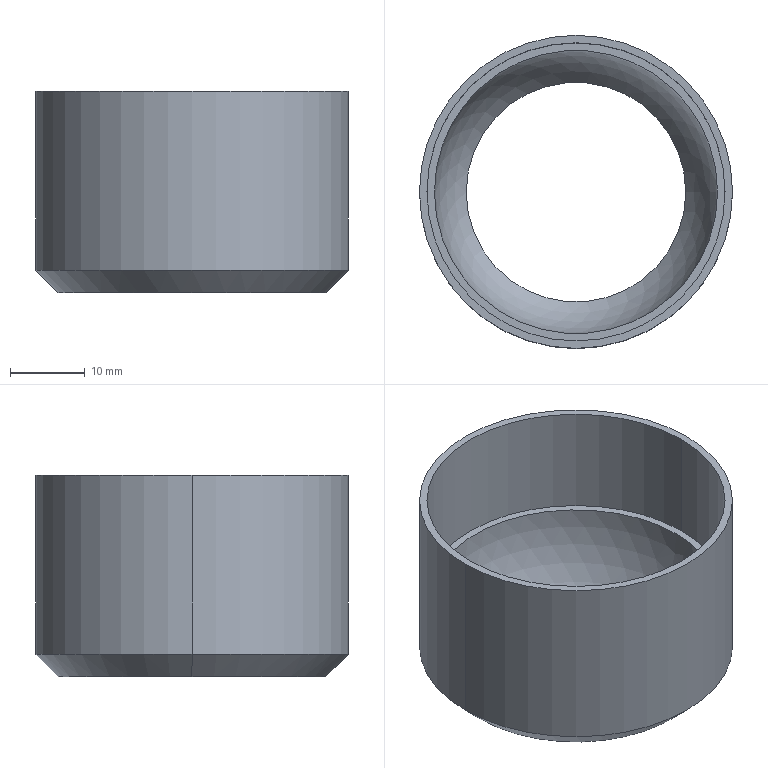Part | SolidWorks | features ICE 5, Chamfer 1, Extrusion 1, RevCut 1 | 1 solid | 10 faces | box 42 x 42 x 27 mm | volume 6192 mm3 | cylinder 4 | plane 3 | cone 2 | sphere 1 | commonest cylinder face diameters 40 x2 42 x2
STEP:
#1=CARTESIAN_POINT('',(-18.,0.,18.));
#2=VERTEX_POINT('',#1);
#3=CARTESIAN_POINT('',(18.,0.,18.));
#4=VERTEX_POINT('',#3);
#5=CARTESIAN_POINT('',(0.,0.,18.));
#6=DIRECTION('',(0.,0.,-1.));
#7=DIRECTION('',(-1.,0.,0.));
#8=AXIS2_PLACEMENT_3D('',#5,#6,#7);
#9=CIRCLE('',#8,18.);
#10=EDGE_CURVE('',#2,#4,#9,.T.);
#11=ORIENTED_EDGE('',*,*,#10,.F.);
#12=CARTESIAN_POINT('',(-21.,0.,21.));
#13=VERTEX_POINT('',#12);
#14=CARTESIAN_POINT('',(-18.,0.,18.));
#15=DIRECTION('',(-0.7071,0.,0.7071));
#16=VECTOR('',#15,1000.);
#17=LINE('',#14,#16);
#18=EDGE_CURVE('',#2,#13,#17,.T.);
#19=ORIENTED_EDGE('',*,*,#18,.T.);
#20=CARTESIAN_POINT('',(21.,0.,21.));
#21=VERTEX_POINT('',#20);
#22=CARTESIAN_POINT('',(0.,0.,21.));
#23=DIRECTION('',(0.,0.,1.));
#24=DIRECTION('',(-1.,0.,0.));
#25=AXIS2_PLACEMENT_3D('',#22,#23,#24);
#26=CIRCLE('',#25,21.);
#27=EDGE_CURVE('',#21,#13,#26,.T.);
#28=ORIENTED_EDGE('',*,*,#27,.F.);
#29=CARTESIAN_POINT('',(18.,0.,18.));
#30=DIRECTION('',(0.7071,0.,0.7071));
#31=VECTOR('',#30,1000.);
#32=LINE('',#29,#31);
#33=EDGE_CURVE('',#4,#21,#32,.T.);
#34=ORIENTED_EDGE('',*,*,#33,.F.);
#35=EDGE_LOOP('',(#11,#19,#28,#34));
#36=FACE_OUTER_BOUND('',#35,.T.);
#37=CARTESIAN_POINT('',(0.,0.,18.));
#38=DIRECTION('',(0.,0.,1.));
#39=DIRECTION('',(1.,0.,0.));
#40=AXIS2_PLACEMENT_3D('',#37,#38,#39);
#41=CONICAL_SURFACE('',#40,18.,0.7854);
#42=ADVANCED_FACE('',(#36),#41,.T.);
#43=CARTESIAN_POINT('',(-20.,0.,30.));
#44=VERTEX_POINT('',#43);
#45=CARTESIAN_POINT('',(20.,0.,30.));
#46=VERTEX_POINT('',#45);
#47=CARTESIAN_POINT('',(0.,0.,30.));
#48=DIRECTION('',(0.,0.,1.));
#49=DIRECTION('',(1.,0.,0.));
#50=AXIS2_PLACEMENT_3D('',#47,#48,#49);
#51=CIRCLE('',#50,20.);
#52=EDGE_CURVE('',#44,#46,#51,.T.);
#53=ORIENTED_EDGE('',*,*,#52,.F.);
#54=CARTESIAN_POINT('',(-20.,0.,45.));
#55=VERTEX_POINT('',#54);
#56=CARTESIAN_POINT('',(-20.,0.,30.));
#57=DIRECTION('',(0.,0.,1.));
#58=VECTOR('',#57,1000.);
#59=LINE('',#56,#58);
#60=EDGE_CURVE('',#44,#55,#59,.T.);
#61=ORIENTED_EDGE('',*,*,#60,.T.);
#62=CARTESIAN_POINT('',(20.,0.,45.));
#63=VERTEX_POINT('',#62);
#64=CARTESIAN_POINT('',(0.,0.,45.));
#65=DIRECTION('',(0.,0.,1.));
#66=DIRECTION('',(1.,0.,0.));
#67=AXIS2_PLACEMENT_3D('',#64,#65,#66);
#68=CIRCLE('',#67,20.);
#69=EDGE_CURVE('',#55,#63,#68,.T.);
#70=ORIENTED_EDGE('',*,*,#69,.T.);
#71=CARTESIAN_POINT('',(20.,0.,30.));
#72=DIRECTION('',(0.,0.,1.));
#73=VECTOR('',#72,1000.);
#74=LINE('',#71,#73);
#75=EDGE_CURVE('',#46,#63,#74,.T.);
#76=ORIENTED_EDGE('',*,*,#75,.F.);
#77=EDGE_LOOP('',(#53,#61,#70,#76));
#78=FACE_OUTER_BOUND('',#77,.T.);
#79=CARTESIAN_POINT('',(0.,0.,30.));
#80=DIRECTION('',(0.,0.,1.));
#81=DIRECTION('',(1.,0.,0.));
#82=AXIS2_PLACEMENT_3D('',#79,#80,#81);
#83=CYLINDRICAL_SURFACE('',#82,20.);
#84=ADVANCED_FACE('',(#78),#83,.F.);
#85=CARTESIAN_POINT('',(21.,0.,45.));
#86=VERTEX_POINT('',#85);
#87=CARTESIAN_POINT('',(-21.,0.,45.));
#88=VERTEX_POINT('',#87);
#89=CARTESIAN_POINT('',(0.,0.,45.));
#90=DIRECTION('',(0.,0.,1.));
#91=DIRECTION('',(1.,0.,0.));
#92=AXIS2_PLACEMENT_3D('',#89,#90,#91);
#93=CIRCLE('',#92,21.);
#94=EDGE_CURVE('',#86,#88,#93,.T.);
#95=ORIENTED_EDGE('',*,*,#94,.F.);
#96=CARTESIAN_POINT('',(21.,0.,45.));
#97=DIRECTION('',(0.,0.,-1.));
#98=VECTOR('',#97,1000.);
#99=LINE('',#96,#98);
#100=EDGE_CURVE('',#86,#21,#99,.T.);
#101=ORIENTED_EDGE('',*,*,#100,.T.);
#102=ORIENTED_EDGE('',*,*,#27,.T.);
#103=CARTESIAN_POINT('',(-21.,0.,45.));
#104=DIRECTION('',(0.,0.,-1.));
#105=VECTOR('',#104,1000.);
#106=LINE('',#103,#105);
#107=EDGE_CURVE('',#88,#13,#106,.T.);
#108=ORIENTED_EDGE('',*,*,#107,.F.);
#109=EDGE_LOOP('',(#95,#101,#102,#108));
#110=FACE_OUTER_BOUND('',#109,.T.);
#111=CARTESIAN_POINT('',(0.,0.,45.));
#112=DIRECTION('',(0.,0.,-1.));
#113=DIRECTION('',(-1.,0.,0.));
#114=AXIS2_PLACEMENT_3D('',#111,#112,#113);
#115=CYLINDRICAL_SURFACE('',#114,21.);
#116=ADVANCED_FACE('',(#110),#115,.T.);
#117=ORIENTED_EDGE('',*,*,#100,.F.);
#118=CARTESIAN_POINT('',(0.,0.,45.));
#119=DIRECTION('',(0.,0.,1.));
#120=DIRECTION('',(1.,0.,0.));
#121=AXIS2_PLACEMENT_3D('',#118,#119,#120);
#122=CIRCLE('',#121,21.);
#123=EDGE_CURVE('',#88,#86,#122,.T.);
#124=ORIENTED_EDGE('',*,*,#123,.F.);
#125=ORIENTED_EDGE('',*,*,#107,.T.);
#126=CARTESIAN_POINT('',(0.,0.,21.));
#127=DIRECTION('',(0.,0.,1.));
#128=DIRECTION('',(-1.,0.,0.));
#129=AXIS2_PLACEMENT_3D('',#126,#127,#128);
#130=CIRCLE('',#129,21.);
#131=EDGE_CURVE('',#13,#21,#130,.T.);
#132=ORIENTED_EDGE('',*,*,#131,.T.);
#133=EDGE_LOOP('',(#117,#124,#125,#132));
#134=FACE_OUTER_BOUND('',#133,.T.);
#135=CARTESIAN_POINT('',(0.,0.,45.));
#136=DIRECTION('',(0.,0.,-1.));
#137=DIRECTION('',(-1.,0.,0.));
#138=AXIS2_PLACEMENT_3D('',#135,#136,#137);
#139=CYLINDRICAL_SURFACE('',#138,21.);
#140=ADVANCED_FACE('',(#134),#139,.T.);
#141=CARTESIAN_POINT('',(19.,0.,30.));
#142=VERTEX_POINT('',#141);
#143=CARTESIAN_POINT('',(-19.,0.,30.));
#144=VERTEX_POINT('',#143);
#145=CARTESIAN_POINT('',(0.,0.,30.));
#146=DIRECTION('',(0.,0.,-1.));
#147=DIRECTION('',(1.,0.,0.));
#148=AXIS2_PLACEMENT_3D('',#145,#146,#147);
#149=CIRCLE('',#148,19.);
#150=EDGE_CURVE('',#142,#144,#149,.T.);
#151=ORIENTED_EDGE('',*,*,#150,.F.);
#152=CARTESIAN_POINT('',(0.,0.,30.));
#153=DIRECTION('',(0.,0.,-1.));
#154=DIRECTION('',(1.,0.,0.));
#155=AXIS2_PLACEMENT_3D('',#152,#153,#154);
#156=CIRCLE('',#155,19.);
#157=EDGE_CURVE('',#144,#142,#156,.T.);
#158=ORIENTED_EDGE('',*,*,#157,.F.);
#159=EDGE_LOOP('',(#151,#158));
#160=FACE_OUTER_BOUND('',#159,.T.);
#161=CARTESIAN_POINT('',(-14.731,0.,18.));
#162=VERTEX_POINT('',#161);
#163=CARTESIAN_POINT('',(14.731,0.,18.));
#164=VERTEX_POINT('',#163);
#165=CARTESIAN_POINT('',(0.,0.,18.));
#166=DIRECTION('',(0.,0.,1.));
#167=DIRECTION('',(-1.,0.,0.));
#168=AXIS2_PLACEMENT_3D('',#165,#166,#167);
#169=CIRCLE('',#168,14.731);
#170=EDGE_CURVE('',#162,#164,#169,.T.);
#171=ORIENTED_EDGE('',*,*,#170,.F.);
#172=CARTESIAN_POINT('',(0.,0.,18.));
#173=DIRECTION('',(0.,0.,1.));
#174=DIRECTION('',(-1.,0.,0.));
#175=AXIS2_PLACEMENT_3D('',#172,#173,#174);
#176=CIRCLE('',#175,14.731);
#177=EDGE_CURVE('',#164,#162,#176,.T.);
#178=ORIENTED_EDGE('',*,*,#177,.F.);
#179=EDGE_LOOP('',(#171,#178));
#180=FACE_BOUND('',#179,.T.);
#181=CARTESIAN_POINT('',(0.,0.,30.));
#182=DIRECTION('',(0.,0.,-1.));
#183=DIRECTION('',(0.,-1.,0.));
#184=AXIS2_PLACEMENT_3D('',#181,#182,#183);
#185=SPHERICAL_SURFACE('',#184,19.);
#186=ADVANCED_FACE('',(#160,#180),#185,.F.);
#187=CARTESIAN_POINT('',(0.,0.,45.));
#188=DIRECTION('',(0.,0.,1.));
#189=DIRECTION('',(1.,0.,0.));
#190=AXIS2_PLACEMENT_3D('',#187,#188,#189);
#191=CIRCLE('',#190,20.);
#192=EDGE_CURVE('',#63,#55,#191,.T.);
#193=ORIENTED_EDGE('',*,*,#192,.F.);
#194=ORIENTED_EDGE('',*,*,#69,.F.);
#195=EDGE_LOOP('',(#193,#194));
#196=FACE_BOUND('',#195,.T.);
#197=ORIENTED_EDGE('',*,*,#123,.T.);
#198=ORIENTED_EDGE('',*,*,#94,.T.);
#199=EDGE_LOOP('',(#197,#198));
#200=FACE_OUTER_BOUND('',#199,.T.);
#201=CARTESIAN_POINT('',(0.,0.,45.));
#202=DIRECTION('',(0.,0.,1.));
#203=DIRECTION('',(1.,0.,0.));
#204=AXIS2_PLACEMENT_3D('',#201,#202,#203);
#205=PLANE('',#204);
#206=ADVANCED_FACE('',(#196,#200),#205,.T.);
#207=CARTESIAN_POINT('',(0.,0.,30.));
#208=DIRECTION('',(0.,0.,1.));
#209=DIRECTION('',(1.,0.,0.));
#210=AXIS2_PLACEMENT_3D('',#207,#208,#209);
#211=CIRCLE('',#210,20.);
#212=EDGE_CURVE('',#46,#44,#211,.T.);
#213=ORIENTED_EDGE('',*,*,#212,.T.);
#214=ORIENTED_EDGE('',*,*,#52,.T.);
#215=EDGE_LOOP('',(#213,#214));
#216=FACE_OUTER_BOUND('',#215,.T.);
#217=ORIENTED_EDGE('',*,*,#150,.T.);
#218=ORIENTED_EDGE('',*,*,#157,.T.);
#219=EDGE_LOOP('',(#217,#218));
#220=FACE_BOUND('',#219,.T.);
#221=CARTESIAN_POINT('',(0.,0.,30.));
#222=DIRECTION('',(0.,0.,1.));
#223=DIRECTION('',(1.,0.,0.));
#224=AXIS2_PLACEMENT_3D('',#221,#222,#223);
#225=PLANE('',#224);
#226=ADVANCED_FACE('',(#216,#220),#225,.T.);
#227=ORIENTED_EDGE('',*,*,#60,.F.);
#228=ORIENTED_EDGE('',*,*,#212,.F.);
#229=ORIENTED_EDGE('',*,*,#75,.T.);
#230=ORIENTED_EDGE('',*,*,#192,.T.);
#231=EDGE_LOOP('',(#227,#228,#229,#230));
#232=FACE_OUTER_BOUND('',#231,.T.);
#233=CARTESIAN_POINT('',(0.,0.,30.));
#234=DIRECTION('',(0.,0.,1.));
#235=DIRECTION('',(1.,0.,0.));
#236=AXIS2_PLACEMENT_3D('',#233,#234,#235);
#237=CYLINDRICAL_SURFACE('',#236,20.);
#238=ADVANCED_FACE('',(#232),#237,.F.);
#239=CARTESIAN_POINT('',(0.,0.,18.));
#240=DIRECTION('',(0.,0.,-1.));
#241=DIRECTION('',(-1.,0.,0.));
#242=AXIS2_PLACEMENT_3D('',#239,#240,#241);
#243=CIRCLE('',#242,18.);
#244=EDGE_CURVE('',#4,#2,#243,.T.);
#245=ORIENTED_EDGE('',*,*,#244,.T.);
#246=ORIENTED_EDGE('',*,*,#10,.T.);
#247=EDGE_LOOP('',(#245,#246));
#248=FACE_OUTER_BOUND('',#247,.T.);
#249=ORIENTED_EDGE('',*,*,#170,.T.);
#250=ORIENTED_EDGE('',*,*,#177,.T.);
#251=EDGE_LOOP('',(#249,#250));
#252=FACE_BOUND('',#251,.T.);
#253=CARTESIAN_POINT('',(0.,0.,18.));
#254=DIRECTION('',(0.,0.,-1.));
#255=DIRECTION('',(-1.,0.,0.));
#256=AXIS2_PLACEMENT_3D('',#253,#254,#255);
#257=PLANE('',#256);
#258=ADVANCED_FACE('',(#248,#252),#257,.T.);
#259=ORIENTED_EDGE('',*,*,#18,.F.);
#260=ORIENTED_EDGE('',*,*,#244,.F.);
#261=ORIENTED_EDGE('',*,*,#33,.T.);
#262=ORIENTED_EDGE('',*,*,#131,.F.);
#263=EDGE_LOOP('',(#259,#260,#261,#262));
#264=FACE_OUTER_BOUND('',#263,.T.);
#265=CARTESIAN_POINT('',(0.,0.,18.));
#266=DIRECTION('',(0.,0.,1.));
#267=DIRECTION('',(1.,0.,0.));
#268=AXIS2_PLACEMENT_3D('',#265,#266,#267);
#269=CONICAL_SURFACE('',#268,18.,0.7854);
#270=ADVANCED_FACE('',(#264),#269,.T.);
#271=CLOSED_SHELL('',(#42,#84,#116,#140,#186,#206,#226,#238,#258,#270));
#272=MANIFOLD_SOLID_BREP('',#271);
#273=CARTESIAN_POINT('',(0.,0.,0.));
#274=DIRECTION('',(0.,0.,1.));
#275=DIRECTION('',(1.,0.,0.));
#276=AXIS2_PLACEMENT_3D('',#273,#274,#275);
#277=(LENGTH_UNIT()NAMED_UNIT(*)SI_UNIT(.MILLI.,.METRE.));
#278=UNCERTAINTY_MEASURE_WITH_UNIT(LENGTH_MEASURE(0.00001),#277,'','');
#279=(NAMED_UNIT(*)PLANE_ANGLE_UNIT()SI_UNIT($,.RADIAN.));
#280=(NAMED_UNIT(*)SI_UNIT($,.STERADIAN.)SOLID_ANGLE_UNIT());
#281=(GEOMETRIC_REPRESENTATION_CONTEXT(3)GLOBAL_UNCERTAINTY_ASSIGNED_CONTEXT((#278))GLOBAL_UNIT_ASSIGNED_CONTEXT((#277,#279,#280))REPRESENTATION_CONTEXT('',''));
#282=ADVANCED_BREP_SHAPE_REPRESENTATION('',(#272,#276),#281);